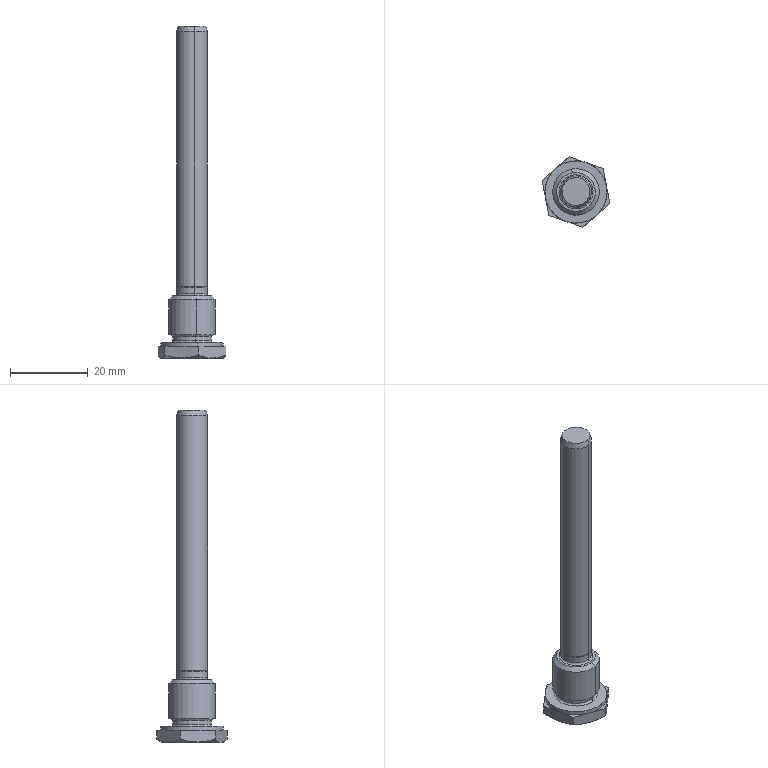Part | SolidWorks | features BaseBody 1 | 1 solid | 46 faces | box 17.462 x 18.14 x 85.5 mm | volume 5617 mm3 | plane 17 | cone 11 | cylinder 10 | torus 8 | commonest cylinder face diameters 7.8 x2 8 x2 10 x2 12 x2 16 x2
STEP:
#1=CARTESIAN_POINT('',(389.341,188.927,-32.5));
#2=VERTEX_POINT('',#1);
#3=CARTESIAN_POINT('',(390.859,181.073,-32.5));
#4=VERTEX_POINT('',#3);
#5=CARTESIAN_POINT('',(390.1,185.,-32.5));
#6=DIRECTION('',(0.,0.,-1.));
#7=DIRECTION('',(0.1897,-0.9818,0.));
#8=AXIS2_PLACEMENT_3D('',#5,#6,#7);
#9=CIRCLE('',#8,4.);
#10=EDGE_CURVE('',#2,#4,#9,.T.);
#11=ORIENTED_EDGE('',*,*,#10,.T.);
#12=CARTESIAN_POINT('',(390.84,181.171,-32.8));
#13=VERTEX_POINT('',#12);
#14=CARTESIAN_POINT('',(390.935,180.68,-32.8));
#15=DIRECTION('',(-0.9818,-0.1897,0.));
#16=DIRECTION('',(0.1897,-0.9818,0.));
#17=AXIS2_PLACEMENT_3D('',#14,#15,#16);
#18=CIRCLE('',#17,0.5);
#19=EDGE_CURVE('',#4,#13,#18,.T.);
#20=ORIENTED_EDGE('',*,*,#19,.T.);
#21=CARTESIAN_POINT('',(389.36,188.829,-32.8));
#22=VERTEX_POINT('',#21);
#23=CARTESIAN_POINT('',(390.1,185.,-32.8));
#24=DIRECTION('',(0.,0.,-1.));
#25=DIRECTION('',(-0.1897,0.9818,0.));
#26=AXIS2_PLACEMENT_3D('',#23,#24,#25);
#27=CIRCLE('',#26,3.9);
#28=EDGE_CURVE('',#22,#13,#27,.T.);
#29=ORIENTED_EDGE('',*,*,#28,.F.);
#30=CARTESIAN_POINT('',(389.265,189.32,-32.8));
#31=DIRECTION('',(0.9818,0.1897,0.));
#32=DIRECTION('',(-0.1897,0.9818,0.));
#33=AXIS2_PLACEMENT_3D('',#30,#31,#32);
#34=CIRCLE('',#33,0.5);
#35=EDGE_CURVE('',#2,#22,#34,.T.);
#36=ORIENTED_EDGE('',*,*,#35,.F.);
#37=EDGE_LOOP('',(#11,#20,#29,#36));
#38=FACE_OUTER_BOUND('',#37,.T.);
#39=CARTESIAN_POINT('',(390.1,185.,-32.8));
#40=DIRECTION('',(0.,0.,1.));
#41=DIRECTION('',(-0.1897,0.9818,0.));
#42=AXIS2_PLACEMENT_3D('',#39,#40,#41);
#43=TOROIDAL_SURFACE('',#42,4.4,0.5);
#44=ADVANCED_FACE('',(#38),#43,.F.);
#45=CARTESIAN_POINT('',(390.84,181.171,-34.5));
#46=VERTEX_POINT('',#45);
#47=CARTESIAN_POINT('',(389.36,188.829,-34.5));
#48=VERTEX_POINT('',#47);
#49=CARTESIAN_POINT('',(390.1,185.,-34.5));
#50=DIRECTION('',(0.,0.,1.));
#51=DIRECTION('',(-0.1897,0.9818,0.));
#52=AXIS2_PLACEMENT_3D('',#49,#50,#51);
#53=CIRCLE('',#52,3.9);
#54=EDGE_CURVE('',#46,#48,#53,.T.);
#55=ORIENTED_EDGE('',*,*,#54,.F.);
#56=CARTESIAN_POINT('',(390.935,180.68,-35.));
#57=VERTEX_POINT('',#56);
#58=CARTESIAN_POINT('',(390.935,180.68,-34.5));
#59=DIRECTION('',(-0.9818,-0.1897,0.));
#60=DIRECTION('',(0.1897,-0.9818,0.));
#61=AXIS2_PLACEMENT_3D('',#58,#59,#60);
#62=CIRCLE('',#61,0.5);
#63=EDGE_CURVE('',#46,#57,#62,.T.);
#64=ORIENTED_EDGE('',*,*,#63,.T.);
#65=CARTESIAN_POINT('',(389.265,189.32,-35.));
#66=VERTEX_POINT('',#65);
#67=CARTESIAN_POINT('',(390.1,185.,-35.));
#68=DIRECTION('',(0.,0.,-1.));
#69=DIRECTION('',(-0.1897,0.9818,0.));
#70=AXIS2_PLACEMENT_3D('',#67,#68,#69);
#71=CIRCLE('',#70,4.4);
#72=EDGE_CURVE('',#66,#57,#71,.T.);
#73=ORIENTED_EDGE('',*,*,#72,.F.);
#74=CARTESIAN_POINT('',(389.265,189.32,-34.5));
#75=DIRECTION('',(0.9818,0.1897,0.));
#76=DIRECTION('',(-0.1897,0.9818,0.));
#77=AXIS2_PLACEMENT_3D('',#74,#75,#76);
#78=CIRCLE('',#77,0.5);
#79=EDGE_CURVE('',#48,#66,#78,.T.);
#80=ORIENTED_EDGE('',*,*,#79,.F.);
#81=EDGE_LOOP('',(#55,#64,#73,#80));
#82=FACE_OUTER_BOUND('',#81,.T.);
#83=CARTESIAN_POINT('',(390.1,185.,-34.5));
#84=DIRECTION('',(0.,0.,1.));
#85=DIRECTION('',(-0.1897,0.9818,0.));
#86=AXIS2_PLACEMENT_3D('',#83,#84,#85);
#87=TOROIDAL_SURFACE('',#86,4.4,0.5);
#88=ADVANCED_FACE('',(#82),#87,.F.);
#89=CARTESIAN_POINT('',(391.143,179.6,-45.));
#90=VERTEX_POINT('',#89);
#91=CARTESIAN_POINT('',(389.057,190.4,-45.));
#92=VERTEX_POINT('',#91);
#93=CARTESIAN_POINT('',(390.1,185.,-45.));
#94=DIRECTION('',(0.,0.,1.));
#95=DIRECTION('',(-0.1897,0.9818,0.));
#96=AXIS2_PLACEMENT_3D('',#93,#94,#95);
#97=CIRCLE('',#96,5.5);
#98=EDGE_CURVE('',#90,#92,#97,.T.);
#99=ORIENTED_EDGE('',*,*,#98,.F.);
#100=CARTESIAN_POINT('',(391.048,180.091,-45.5));
#101=VERTEX_POINT('',#100);
#102=CARTESIAN_POINT('',(391.143,179.6,-45.5));
#103=DIRECTION('',(-0.9818,-0.1897,0.));
#104=DIRECTION('',(0.1897,-0.9818,0.));
#105=AXIS2_PLACEMENT_3D('',#102,#103,#104);
#106=CIRCLE('',#105,0.5);
#107=EDGE_CURVE('',#90,#101,#106,.T.);
#108=ORIENTED_EDGE('',*,*,#107,.T.);
#109=CARTESIAN_POINT('',(389.152,189.909,-45.5));
#110=VERTEX_POINT('',#109);
#111=CARTESIAN_POINT('',(390.1,185.,-45.5));
#112=DIRECTION('',(0.,0.,-1.));
#113=DIRECTION('',(-0.1897,0.9818,0.));
#114=AXIS2_PLACEMENT_3D('',#111,#112,#113);
#115=CIRCLE('',#114,5.);
#116=EDGE_CURVE('',#110,#101,#115,.T.);
#117=ORIENTED_EDGE('',*,*,#116,.F.);
#118=CARTESIAN_POINT('',(389.057,190.4,-45.5));
#119=DIRECTION('',(0.9818,0.1897,0.));
#120=DIRECTION('',(-0.1897,0.9818,0.));
#121=AXIS2_PLACEMENT_3D('',#118,#119,#120);
#122=CIRCLE('',#121,0.5);
#123=EDGE_CURVE('',#92,#110,#122,.T.);
#124=ORIENTED_EDGE('',*,*,#123,.F.);
#125=EDGE_LOOP('',(#99,#108,#117,#124));
#126=FACE_OUTER_BOUND('',#125,.T.);
#127=CARTESIAN_POINT('',(390.1,185.,-45.5));
#128=DIRECTION('',(0.,0.,1.));
#129=DIRECTION('',(-0.1897,0.9818,0.));
#130=AXIS2_PLACEMENT_3D('',#127,#128,#129);
#131=TOROIDAL_SURFACE('',#130,5.5,0.5);
#132=ADVANCED_FACE('',(#126),#131,.F.);
#133=CARTESIAN_POINT('',(391.618,177.145,-51.));
#134=VERTEX_POINT('',#133);
#135=CARTESIAN_POINT('',(387.487,177.439,-51.));
#136=VERTEX_POINT('',#135);
#137=CARTESIAN_POINT('',(390.1,185.,-51.));
#138=DIRECTION('',(0.,0.,-1.));
#139=DIRECTION('',(0.1897,-0.9818,0.));
#140=AXIS2_PLACEMENT_3D('',#137,#138,#139);
#141=CIRCLE('',#140,8.);
#142=EDGE_CURVE('',#134,#136,#141,.T.);
#143=ORIENTED_EDGE('',*,*,#142,.F.);
#144=CARTESIAN_POINT('',(391.852,175.93,-50.285));
#145=VERTEX_POINT('',#144);
#146=CARTESIAN_POINT('',(391.618,177.145,-51.));
#147=DIRECTION('',(0.1643,-0.8503,0.5));
#148=VECTOR('',#147,1000.);
#149=LINE('',#146,#148);
#150=EDGE_CURVE('',#134,#145,#149,.T.);
#151=ORIENTED_EDGE('',*,*,#150,.T.);
#152=CARTESIAN_POINT('',(387.487,177.439,-51.));
#153=CARTESIAN_POINT('',(387.857,177.311,-51.));
#154=CARTESIAN_POINT('',(388.229,177.182,-50.983));
#155=CARTESIAN_POINT('',(388.966,176.928,-50.918));
#156=CARTESIAN_POINT('',(389.331,176.801,-50.869));
#157=CARTESIAN_POINT('',(390.422,176.425,-50.683));
#158=CARTESIAN_POINT('',(391.14,176.176,-50.503));
#159=CARTESIAN_POINT('',(391.852,175.93,-50.285));
#160=B_SPLINE_CURVE_WITH_KNOTS('',3,(#152,#153,#154,#155,#156,#157,#158,#159),.UNSPECIFIED.,.F.,.F.,(4,2,2,4),(0.004674,0.005838,0.007002,0.00933),.UNSPECIFIED.);
#161=EDGE_CURVE('',#136,#145,#160,.T.);
#162=ORIENTED_EDGE('',*,*,#161,.F.);
#163=EDGE_LOOP('',(#143,#151,#162));
#164=FACE_OUTER_BOUND('',#163,.T.);
#165=CARTESIAN_POINT('',(390.1,185.,-51.));
#166=DIRECTION('',(0.,0.,1.));
#167=DIRECTION('',(0.1897,-0.9818,0.));
#168=AXIS2_PLACEMENT_3D('',#165,#166,#167);
#169=CONICAL_SURFACE('',#168,8.,1.047);
#170=ADVANCED_FACE('',(#164),#169,.T.);
#171=CARTESIAN_POINT('',(389.057,190.4,-47.));
#172=VERTEX_POINT('',#171);
#173=CARTESIAN_POINT('',(391.143,179.6,-47.));
#174=VERTEX_POINT('',#173);
#175=CARTESIAN_POINT('',(390.1,185.,-47.));
#176=DIRECTION('',(0.,0.,-1.));
#177=DIRECTION('',(0.1897,-0.9818,0.));
#178=AXIS2_PLACEMENT_3D('',#175,#176,#177);
#179=CIRCLE('',#178,5.5);
#180=EDGE_CURVE('',#172,#174,#179,.T.);
#181=ORIENTED_EDGE('',*,*,#180,.F.);
#182=CARTESIAN_POINT('',(389.152,189.909,-46.5));
#183=VERTEX_POINT('',#182);
#184=CARTESIAN_POINT('',(389.057,190.4,-46.5));
#185=DIRECTION('',(-0.9818,-0.1897,0.));
#186=DIRECTION('',(0.1897,-0.9818,0.));
#187=AXIS2_PLACEMENT_3D('',#184,#185,#186);
#188=CIRCLE('',#187,0.5);
#189=EDGE_CURVE('',#172,#183,#188,.T.);
#190=ORIENTED_EDGE('',*,*,#189,.T.);
#191=CARTESIAN_POINT('',(391.048,180.091,-46.5));
#192=VERTEX_POINT('',#191);
#193=CARTESIAN_POINT('',(390.1,185.,-46.5));
#194=DIRECTION('',(0.,0.,1.));
#195=DIRECTION('',(0.1897,-0.9818,0.));
#196=AXIS2_PLACEMENT_3D('',#193,#194,#195);
#197=CIRCLE('',#196,5.);
#198=EDGE_CURVE('',#192,#183,#197,.T.);
#199=ORIENTED_EDGE('',*,*,#198,.F.);
#200=CARTESIAN_POINT('',(391.143,179.6,-46.5));
#201=DIRECTION('',(0.9818,0.1897,0.));
#202=DIRECTION('',(-0.1897,0.9818,0.));
#203=AXIS2_PLACEMENT_3D('',#200,#201,#202);
#204=CIRCLE('',#203,0.5);
#205=EDGE_CURVE('',#174,#192,#204,.T.);
#206=ORIENTED_EDGE('',*,*,#205,.F.);
#207=EDGE_LOOP('',(#181,#190,#199,#206));
#208=FACE_OUTER_BOUND('',#207,.T.);
#209=CARTESIAN_POINT('',(390.1,185.,-46.5));
#210=DIRECTION('',(0.,0.,-1.));
#211=DIRECTION('',(0.1897,-0.9818,0.));
#212=AXIS2_PLACEMENT_3D('',#209,#210,#211);
#213=TOROIDAL_SURFACE('',#212,5.5,0.5);
#214=ADVANCED_FACE('',(#208),#213,.F.);
#215=CARTESIAN_POINT('',(389.152,189.909,-35.));
#216=VERTEX_POINT('',#215);
#217=CARTESIAN_POINT('',(391.048,180.091,-35.));
#218=VERTEX_POINT('',#217);
#219=CARTESIAN_POINT('',(390.1,185.,-35.));
#220=DIRECTION('',(0.,0.,1.));
#221=DIRECTION('',(-0.1897,0.9818,0.));
#222=AXIS2_PLACEMENT_3D('',#219,#220,#221);
#223=CIRCLE('',#222,5.);
#224=EDGE_CURVE('',#216,#218,#223,.T.);
#225=ORIENTED_EDGE('',*,*,#224,.F.);
#226=CARTESIAN_POINT('',(388.962,190.891,-36.));
#227=VERTEX_POINT('',#226);
#228=CARTESIAN_POINT('',(388.962,190.891,-36.));
#229=DIRECTION('',(-0.1341,0.6943,-0.7071));
#230=VECTOR('',#229,1000.);
#231=LINE('',#228,#230);
#232=EDGE_CURVE('',#216,#227,#231,.T.);
#233=ORIENTED_EDGE('',*,*,#232,.T.);
#234=CARTESIAN_POINT('',(391.238,179.109,-36.));
#235=VERTEX_POINT('',#234);
#236=CARTESIAN_POINT('',(390.1,185.,-36.));
#237=DIRECTION('',(0.,0.,-1.));
#238=DIRECTION('',(-0.1897,0.9818,0.));
#239=AXIS2_PLACEMENT_3D('',#236,#237,#238);
#240=CIRCLE('',#239,6.);
#241=EDGE_CURVE('',#235,#227,#240,.T.);
#242=ORIENTED_EDGE('',*,*,#241,.F.);
#243=CARTESIAN_POINT('',(391.238,179.109,-36.));
#244=DIRECTION('',(0.1341,-0.6943,-0.7071));
#245=VECTOR('',#244,1000.);
#246=LINE('',#243,#245);
#247=EDGE_CURVE('',#218,#235,#246,.T.);
#248=ORIENTED_EDGE('',*,*,#247,.F.);
#249=EDGE_LOOP('',(#225,#233,#242,#248));
#250=FACE_OUTER_BOUND('',#249,.T.);
#251=CARTESIAN_POINT('',(390.1,185.,-36.));
#252=DIRECTION('',(0.,0.,-1.));
#253=DIRECTION('',(0.1897,-0.9818,0.));
#254=AXIS2_PLACEMENT_3D('',#251,#252,#253);
#255=CONICAL_SURFACE('',#254,6.,0.7854);
#256=ADVANCED_FACE('',(#250),#255,.T.);
#257=CARTESIAN_POINT('',(391.618,177.145,-47.));
#258=VERTEX_POINT('',#257);
#259=CARTESIAN_POINT('',(388.582,192.855,-47.));
#260=VERTEX_POINT('',#259);
#261=CARTESIAN_POINT('',(390.1,185.,-47.));
#262=DIRECTION('',(0.,0.,-1.));
#263=DIRECTION('',(0.1897,-0.9818,0.));
#264=AXIS2_PLACEMENT_3D('',#261,#262,#263);
#265=CIRCLE('',#264,8.);
#266=EDGE_CURVE('',#258,#260,#265,.T.);
#267=ORIENTED_EDGE('',*,*,#266,.T.);
#268=CARTESIAN_POINT('',(388.582,192.855,-48.));
#269=VERTEX_POINT('',#268);
#270=CARTESIAN_POINT('',(388.582,192.855,-51.));
#271=DIRECTION('',(0.,0.,-1.));
#272=VECTOR('',#271,1000.);
#273=LINE('',#270,#272);
#274=EDGE_CURVE('',#260,#269,#273,.T.);
#275=ORIENTED_EDGE('',*,*,#274,.T.);
#276=CARTESIAN_POINT('',(384.858,191.044,-48.));
#277=VERTEX_POINT('',#276);
#278=CARTESIAN_POINT('',(390.1,185.,-48.));
#279=DIRECTION('',(0.,0.,-1.));
#280=DIRECTION('',(0.1897,-0.9818,0.));
#281=AXIS2_PLACEMENT_3D('',#278,#279,#280);
#282=CIRCLE('',#281,8.);
#283=EDGE_CURVE('',#277,#269,#282,.T.);
#284=ORIENTED_EDGE('',*,*,#283,.F.);
#285=CARTESIAN_POINT('',(382.245,183.482,-48.));
#286=VERTEX_POINT('',#285);
#287=CARTESIAN_POINT('',(390.1,185.,-48.));
#288=DIRECTION('',(0.,0.,-1.));
#289=DIRECTION('',(0.1897,-0.9818,0.));
#290=AXIS2_PLACEMENT_3D('',#287,#288,#289);
#291=CIRCLE('',#290,8.);
#292=EDGE_CURVE('',#286,#277,#291,.T.);
#293=ORIENTED_EDGE('',*,*,#292,.F.);
#294=CARTESIAN_POINT('',(387.487,177.439,-48.));
#295=VERTEX_POINT('',#294);
#296=CARTESIAN_POINT('',(390.1,185.,-48.));
#297=DIRECTION('',(0.,0.,-1.));
#298=DIRECTION('',(0.1897,-0.9818,0.));
#299=AXIS2_PLACEMENT_3D('',#296,#297,#298);
#300=CIRCLE('',#299,8.);
#301=EDGE_CURVE('',#295,#286,#300,.T.);
#302=ORIENTED_EDGE('',*,*,#301,.F.);
#303=CARTESIAN_POINT('',(391.618,177.145,-48.));
#304=VERTEX_POINT('',#303);
#305=CARTESIAN_POINT('',(390.1,185.,-48.));
#306=DIRECTION('',(0.,0.,-1.));
#307=DIRECTION('',(0.1897,-0.9818,0.));
#308=AXIS2_PLACEMENT_3D('',#305,#306,#307);
#309=CIRCLE('',#308,8.);
#310=EDGE_CURVE('',#304,#295,#309,.T.);
#311=ORIENTED_EDGE('',*,*,#310,.F.);
#312=CARTESIAN_POINT('',(391.618,177.145,-51.));
#313=DIRECTION('',(0.,0.,-1.));
#314=VECTOR('',#313,1000.);
#315=LINE('',#312,#314);
#316=EDGE_CURVE('',#258,#304,#315,.T.);
#317=ORIENTED_EDGE('',*,*,#316,.F.);
#318=EDGE_LOOP('',(#267,#275,#284,#293,#302,#311,#317));
#319=FACE_OUTER_BOUND('',#318,.T.);
#320=CARTESIAN_POINT('',(390.1,185.,-51.));
#321=DIRECTION('',(0.,0.,-1.));
#322=DIRECTION('',(0.1897,-0.9818,0.));
#323=AXIS2_PLACEMENT_3D('',#320,#321,#322);
#324=CYLINDRICAL_SURFACE('',#323,8.);
#325=ADVANCED_FACE('',(#319),#324,.T.);
#326=CARTESIAN_POINT('',(390.1,185.,-45.5));
#327=DIRECTION('',(0.,0.,-1.));
#328=DIRECTION('',(-0.1897,0.9818,0.));
#329=AXIS2_PLACEMENT_3D('',#326,#327,#328);
#330=CIRCLE('',#329,5.);
#331=EDGE_CURVE('',#101,#110,#330,.T.);
#332=ORIENTED_EDGE('',*,*,#331,.T.);
#333=CARTESIAN_POINT('',(389.152,189.909,-51.));
#334=DIRECTION('',(0.,0.,-1.));
#335=VECTOR('',#334,1000.);
#336=LINE('',#333,#335);
#337=EDGE_CURVE('',#110,#183,#336,.T.);
#338=ORIENTED_EDGE('',*,*,#337,.T.);
#339=CARTESIAN_POINT('',(390.1,185.,-46.5));
#340=DIRECTION('',(0.,0.,1.));
#341=DIRECTION('',(0.1897,-0.9818,0.));
#342=AXIS2_PLACEMENT_3D('',#339,#340,#341);
#343=CIRCLE('',#342,5.);
#344=EDGE_CURVE('',#183,#192,#343,.T.);
#345=ORIENTED_EDGE('',*,*,#344,.T.);
#346=CARTESIAN_POINT('',(391.048,180.091,-51.));
#347=DIRECTION('',(0.,0.,-1.));
#348=VECTOR('',#347,1000.);
#349=LINE('',#346,#348);
#350=EDGE_CURVE('',#101,#192,#349,.T.);
#351=ORIENTED_EDGE('',*,*,#350,.F.);
#352=EDGE_LOOP('',(#332,#338,#345,#351));
#353=FACE_OUTER_BOUND('',#352,.T.);
#354=CARTESIAN_POINT('',(390.1,185.,-51.));
#355=DIRECTION('',(0.,0.,-1.));
#356=DIRECTION('',(0.1897,-0.9818,0.));
#357=AXIS2_PLACEMENT_3D('',#354,#355,#356);
#358=CYLINDRICAL_SURFACE('',#357,5.);
#359=ADVANCED_FACE('',(#353),#358,.T.);
#360=ORIENTED_EDGE('',*,*,#241,.T.);
#361=CARTESIAN_POINT('',(388.962,190.891,-45.));
#362=VERTEX_POINT('',#361);
#363=CARTESIAN_POINT('',(388.962,190.891,-51.));
#364=DIRECTION('',(0.,0.,-1.));
#365=VECTOR('',#364,1000.);
#366=LINE('',#363,#365);
#367=EDGE_CURVE('',#227,#362,#366,.T.);
#368=ORIENTED_EDGE('',*,*,#367,.T.);
#369=CARTESIAN_POINT('',(391.238,179.109,-45.));
#370=VERTEX_POINT('',#369);
#371=CARTESIAN_POINT('',(390.1,185.,-45.));
#372=DIRECTION('',(0.,0.,-1.));
#373=DIRECTION('',(0.1897,-0.9818,0.));
#374=AXIS2_PLACEMENT_3D('',#371,#372,#373);
#375=CIRCLE('',#374,6.);
#376=EDGE_CURVE('',#370,#362,#375,.T.);
#377=ORIENTED_EDGE('',*,*,#376,.F.);
#378=CARTESIAN_POINT('',(391.238,179.109,-51.));
#379=DIRECTION('',(0.,0.,-1.));
#380=VECTOR('',#379,1000.);
#381=LINE('',#378,#380);
#382=EDGE_CURVE('',#235,#370,#381,.T.);
#383=ORIENTED_EDGE('',*,*,#382,.F.);
#384=EDGE_LOOP('',(#360,#368,#377,#383));
#385=FACE_OUTER_BOUND('',#384,.T.);
#386=CARTESIAN_POINT('',(390.1,185.,-51.));
#387=DIRECTION('',(0.,0.,-1.));
#388=DIRECTION('',(0.1897,-0.9818,0.));
#389=AXIS2_PLACEMENT_3D('',#386,#387,#388);
#390=CYLINDRICAL_SURFACE('',#389,6.);
#391=ADVANCED_FACE('',(#385),#390,.T.);
#392=CARTESIAN_POINT('',(390.1,185.,-32.8));
#393=DIRECTION('',(0.,0.,-1.));
#394=DIRECTION('',(-0.1897,0.9818,0.));
#395=AXIS2_PLACEMENT_3D('',#392,#393,#394);
#396=CIRCLE('',#395,3.9);
#397=EDGE_CURVE('',#13,#22,#396,.T.);
#398=ORIENTED_EDGE('',*,*,#397,.T.);
#399=CARTESIAN_POINT('',(389.36,188.829,-51.));
#400=DIRECTION('',(0.,0.,-1.));
#401=VECTOR('',#400,1000.);
#402=LINE('',#399,#401);
#403=EDGE_CURVE('',#22,#48,#402,.T.);
#404=ORIENTED_EDGE('',*,*,#403,.T.);
#405=CARTESIAN_POINT('',(390.1,185.,-34.5));
#406=DIRECTION('',(0.,0.,1.));
#407=DIRECTION('',(-0.1897,0.9818,0.));
#408=AXIS2_PLACEMENT_3D('',#405,#406,#407);
#409=CIRCLE('',#408,3.9);
#410=EDGE_CURVE('',#48,#46,#409,.T.);
#411=ORIENTED_EDGE('',*,*,#410,.T.);
#412=CARTESIAN_POINT('',(390.84,181.171,-51.));
#413=DIRECTION('',(0.,0.,-1.));
#414=VECTOR('',#413,1000.);
#415=LINE('',#412,#414);
#416=EDGE_CURVE('',#13,#46,#415,.T.);
#417=ORIENTED_EDGE('',*,*,#416,.F.);
#418=EDGE_LOOP('',(#398,#404,#411,#417));
#419=FACE_OUTER_BOUND('',#418,.T.);
#420=CARTESIAN_POINT('',(390.1,185.,-51.));
#421=DIRECTION('',(0.,0.,-1.));
#422=DIRECTION('',(0.1897,-0.9818,0.));
#423=AXIS2_PLACEMENT_3D('',#420,#421,#422);
#424=CYLINDRICAL_SURFACE('',#423,3.9);
#425=ADVANCED_FACE('',(#419),#424,.T.);
#426=CARTESIAN_POINT('',(390.859,181.073,33.));
#427=VERTEX_POINT('',#426);
#428=CARTESIAN_POINT('',(389.341,188.927,33.));
#429=VERTEX_POINT('',#428);
#430=CARTESIAN_POINT('',(390.1,185.,33.));
#431=DIRECTION('',(0.,0.,-1.));
#432=DIRECTION('',(0.1897,-0.9818,0.));
#433=AXIS2_PLACEMENT_3D('',#430,#431,#432);
#434=CIRCLE('',#433,4.);
#435=EDGE_CURVE('',#427,#429,#434,.T.);
#436=ORIENTED_EDGE('',*,*,#435,.T.);
#437=CARTESIAN_POINT('',(389.341,188.927,-51.));
#438=DIRECTION('',(0.,0.,-1.));
#439=VECTOR('',#438,1000.);
#440=LINE('',#437,#439);
#441=EDGE_CURVE('',#429,#2,#440,.T.);
#442=ORIENTED_EDGE('',*,*,#441,.T.);
#443=CARTESIAN_POINT('',(390.1,185.,-32.5));
#444=DIRECTION('',(0.,0.,-1.));
#445=DIRECTION('',(0.1897,-0.9818,0.));
#446=AXIS2_PLACEMENT_3D('',#443,#444,#445);
#447=CIRCLE('',#446,4.);
#448=EDGE_CURVE('',#4,#2,#447,.T.);
#449=ORIENTED_EDGE('',*,*,#448,.F.);
#450=CARTESIAN_POINT('',(390.859,181.073,-51.));
#451=DIRECTION('',(0.,0.,-1.));
#452=VECTOR('',#451,1000.);
#453=LINE('',#450,#452);
#454=EDGE_CURVE('',#427,#4,#453,.T.);
#455=ORIENTED_EDGE('',*,*,#454,.F.);
#456=EDGE_LOOP('',(#436,#442,#449,#455));
#457=FACE_OUTER_BOUND('',#456,.T.);
#458=CARTESIAN_POINT('',(390.1,185.,-51.));
#459=DIRECTION('',(0.,0.,-1.));
#460=DIRECTION('',(0.1897,-0.9818,0.));
#461=AXIS2_PLACEMENT_3D('',#458,#459,#460);
#462=CYLINDRICAL_SURFACE('',#461,4.);
#463=ADVANCED_FACE('',(#457),#462,.T.);
#464=CARTESIAN_POINT('',(390.783,181.467,34.5));
#465=VERTEX_POINT('',#464);
#466=CARTESIAN_POINT('',(389.417,188.533,34.5));
#467=VERTEX_POINT('',#466);
#468=CARTESIAN_POINT('',(390.1,185.,34.5));
#469=DIRECTION('',(0.,0.,-1.));
#470=DIRECTION('',(0.1897,-0.9818,0.));
#471=AXIS2_PLACEMENT_3D('',#468,#469,#470);
#472=CIRCLE('',#471,3.598);
#473=EDGE_CURVE('',#465,#467,#472,.T.);
#474=ORIENTED_EDGE('',*,*,#473,.T.);
#475=CARTESIAN_POINT('',(389.417,188.533,34.5));
#476=DIRECTION('',(-0.0491,0.2541,-0.9659));
#477=VECTOR('',#476,1000.);
#478=LINE('',#475,#477);
#479=EDGE_CURVE('',#467,#429,#478,.T.);
#480=ORIENTED_EDGE('',*,*,#479,.T.);
#481=ORIENTED_EDGE('',*,*,#435,.F.);
#482=CARTESIAN_POINT('',(390.783,181.467,34.5));
#483=DIRECTION('',(0.0491,-0.2541,-0.9659));
#484=VECTOR('',#483,1000.);
#485=LINE('',#482,#484);
#486=EDGE_CURVE('',#465,#427,#485,.T.);
#487=ORIENTED_EDGE('',*,*,#486,.F.);
#488=EDGE_LOOP('',(#474,#480,#481,#487));
#489=FACE_OUTER_BOUND('',#488,.T.);
#490=CARTESIAN_POINT('',(390.1,185.,34.5));
#491=DIRECTION('',(0.,0.,-1.));
#492=DIRECTION('',(0.1897,-0.9818,0.));
#493=AXIS2_PLACEMENT_3D('',#490,#491,#492);
#494=CONICAL_SURFACE('',#493,3.598,0.2618);
#495=ADVANCED_FACE('',(#489),#494,.T.);
#496=CARTESIAN_POINT('',(391.852,175.93,-48.));
#497=VERTEX_POINT('',#496);
#498=CARTESIAN_POINT('',(391.852,175.93,-48.));
#499=DIRECTION('',(0.,0.,-1.));
#500=VECTOR('',#499,1000.);
#501=LINE('',#498,#500);
#502=EDGE_CURVE('',#497,#145,#501,.T.);
#503=ORIENTED_EDGE('',*,*,#502,.T.);
#504=CARTESIAN_POINT('',(395.342,178.956,-51.));
#505=VERTEX_POINT('',#504);
#506=CARTESIAN_POINT('',(391.852,175.93,-50.285));
#507=CARTESIAN_POINT('',(392.423,176.425,-50.504));
#508=CARTESIAN_POINT('',(392.998,176.924,-50.683));
#509=CARTESIAN_POINT('',(394.16,177.932,-50.932));
#510=CARTESIAN_POINT('',(394.747,178.441,-51.));
#511=CARTESIAN_POINT('',(395.342,178.956,-51.));
#512=B_SPLINE_CURVE_WITH_KNOTS('',3,(#506,#507,#508,#509,#510,#511),.UNSPECIFIED.,.F.,.F.,(4,2,4),(0.000000238,0.002337,0.004674),.UNSPECIFIED.);
#513=EDGE_CURVE('',#145,#505,#512,.T.);
#514=ORIENTED_EDGE('',*,*,#513,.T.);
#515=CARTESIAN_POINT('',(398.831,181.983,-50.285));
#516=VERTEX_POINT('',#515);
#517=CARTESIAN_POINT('',(395.342,178.956,-51.));
#518=CARTESIAN_POINT('',(395.638,179.213,-51.));
#519=CARTESIAN_POINT('',(395.935,179.471,-50.983));
#520=CARTESIAN_POINT('',(396.524,179.981,-50.918));
#521=CARTESIAN_POINT('',(396.816,180.235,-50.869));
#522=CARTESIAN_POINT('',(397.687,180.991,-50.683));
#523=CARTESIAN_POINT('',(398.262,181.489,-50.503));
#524=CARTESIAN_POINT('',(398.831,181.983,-50.285));
#525=B_SPLINE_CURVE_WITH_KNOTS('',3,(#517,#518,#519,#520,#521,#522,#523,#524),.UNSPECIFIED.,.F.,.F.,(4,2,2,4),(0.004674,0.005838,0.007002,0.00933),.UNSPECIFIED.);
#526=EDGE_CURVE('',#505,#516,#525,.T.);
#527=ORIENTED_EDGE('',*,*,#526,.T.);
#528=CARTESIAN_POINT('',(398.831,181.983,-48.));
#529=VERTEX_POINT('',#528);
#530=CARTESIAN_POINT('',(398.831,181.983,-48.));
#531=DIRECTION('',(0.,0.,-1.));
#532=VECTOR('',#531,1000.);
#533=LINE('',#530,#532);
#534=EDGE_CURVE('',#529,#516,#533,.T.);
#535=ORIENTED_EDGE('',*,*,#534,.F.);
#536=CARTESIAN_POINT('',(395.342,178.956,-48.));
#537=VERTEX_POINT('',#536);
#538=CARTESIAN_POINT('',(398.831,181.983,-48.));
#539=DIRECTION('',(-0.7555,-0.6552,0.));
#540=VECTOR('',#539,1000.);
#541=LINE('',#538,#540);
#542=EDGE_CURVE('',#529,#537,#541,.T.);
#543=ORIENTED_EDGE('',*,*,#542,.T.);
#544=CARTESIAN_POINT('',(398.831,181.983,-48.));
#545=DIRECTION('',(-0.7555,-0.6552,0.));
#546=VECTOR('',#545,1000.);
#547=LINE('',#544,#546);
#548=EDGE_CURVE('',#537,#497,#547,.T.);
#549=ORIENTED_EDGE('',*,*,#548,.T.);
#550=EDGE_LOOP('',(#503,#514,#527,#535,#543,#549));
#551=FACE_OUTER_BOUND('',#550,.T.);
#552=CARTESIAN_POINT('',(398.831,181.983,-48.));
#553=DIRECTION('',(0.6552,-0.7555,0.));
#554=DIRECTION('',(-0.7555,-0.6552,0.));
#555=AXIS2_PLACEMENT_3D('',#552,#553,#554);
#556=PLANE('',#555);
#557=ADVANCED_FACE('',(#551),#556,.T.);
#558=ORIENTED_EDGE('',*,*,#534,.T.);
#559=CARTESIAN_POINT('',(397.955,186.518,-51.));
#560=VERTEX_POINT('',#559);
#561=CARTESIAN_POINT('',(398.831,181.983,-50.285));
#562=CARTESIAN_POINT('',(398.689,182.716,-50.501));
#563=CARTESIAN_POINT('',(398.546,183.459,-50.681));
#564=CARTESIAN_POINT('',(398.326,184.594,-50.868));
#565=CARTESIAN_POINT('',(398.253,184.976,-50.917));
#566=CARTESIAN_POINT('',(398.104,185.747,-50.983));
#567=CARTESIAN_POINT('',(398.029,186.134,-51.));
#568=CARTESIAN_POINT('',(397.955,186.518,-51.));
#569=B_SPLINE_CURVE_WITH_KNOTS('',3,(#561,#562,#563,#564,#565,#566,#567,#568),.UNSPECIFIED.,.F.,.F.,(4,2,2,4),(0.02201,0.02435,0.02552,0.02669),.UNSPECIFIED.);
#570=EDGE_CURVE('',#516,#560,#569,.T.);
#571=ORIENTED_EDGE('',*,*,#570,.T.);
#572=CARTESIAN_POINT('',(397.079,191.052,-50.285));
#573=VERTEX_POINT('',#572);
#574=CARTESIAN_POINT('',(397.955,186.518,-51.));
#575=CARTESIAN_POINT('',(397.806,187.285,-51.));
#576=CARTESIAN_POINT('',(397.659,188.046,-50.933));
#577=CARTESIAN_POINT('',(397.367,189.559,-50.684));
#578=CARTESIAN_POINT('',(397.221,190.314,-50.503));
#579=CARTESIAN_POINT('',(397.079,191.052,-50.285));
#580=B_SPLINE_CURVE_WITH_KNOTS('',3,(#574,#575,#576,#577,#578,#579),.UNSPECIFIED.,.F.,.F.,(4,2,4),(0.02669,0.02903,0.03137),.UNSPECIFIED.);
#581=EDGE_CURVE('',#560,#573,#580,.T.);
#582=ORIENTED_EDGE('',*,*,#581,.T.);
#583=CARTESIAN_POINT('',(397.079,191.052,-48.));
#584=VERTEX_POINT('',#583);
#585=CARTESIAN_POINT('',(397.079,191.052,-48.));
#586=DIRECTION('',(0.,0.,-1.));
#587=VECTOR('',#586,1000.);
#588=LINE('',#585,#587);
#589=EDGE_CURVE('',#584,#573,#588,.T.);
#590=ORIENTED_EDGE('',*,*,#589,.F.);
#591=CARTESIAN_POINT('',(397.955,186.518,-48.));
#592=VERTEX_POINT('',#591);
#593=CARTESIAN_POINT('',(397.079,191.052,-48.));
#594=DIRECTION('',(0.1897,-0.9818,0.));
#595=VECTOR('',#594,1000.);
#596=LINE('',#593,#595);
#597=EDGE_CURVE('',#584,#592,#596,.T.);
#598=ORIENTED_EDGE('',*,*,#597,.T.);
#599=CARTESIAN_POINT('',(397.079,191.052,-48.));
#600=DIRECTION('',(0.1897,-0.9818,0.));
#601=VECTOR('',#600,1000.);
#602=LINE('',#599,#601);
#603=EDGE_CURVE('',#592,#529,#602,.T.);
#604=ORIENTED_EDGE('',*,*,#603,.T.);
#605=EDGE_LOOP('',(#558,#571,#582,#590,#598,#604));
#606=FACE_OUTER_BOUND('',#605,.T.);
#607=CARTESIAN_POINT('',(397.079,191.052,-48.));
#608=DIRECTION('',(0.9818,0.1897,0.));
#609=DIRECTION('',(0.1897,-0.9818,0.));
#610=AXIS2_PLACEMENT_3D('',#607,#608,#609);
#611=PLANE('',#610);
#612=ADVANCED_FACE('',(#606),#611,.T.);
#613=ORIENTED_EDGE('',*,*,#589,.T.);
#614=CARTESIAN_POINT('',(392.713,192.561,-51.));
#615=VERTEX_POINT('',#614);
#616=CARTESIAN_POINT('',(397.079,191.052,-50.285));
#617=CARTESIAN_POINT('',(396.364,191.299,-50.504));
#618=CARTESIAN_POINT('',(395.645,191.548,-50.683));
#619=CARTESIAN_POINT('',(394.191,192.05,-50.932));
#620=CARTESIAN_POINT('',(393.457,192.304,-51.));
#621=CARTESIAN_POINT('',(392.713,192.561,-51.));
#622=B_SPLINE_CURVE_WITH_KNOTS('',3,(#616,#617,#618,#619,#620,#621),.UNSPECIFIED.,.F.,.F.,(4,2,4),(0.000000238,0.002337,0.004674),.UNSPECIFIED.);
#623=EDGE_CURVE('',#573,#615,#622,.T.);
#624=ORIENTED_EDGE('',*,*,#623,.T.);
#625=CARTESIAN_POINT('',(388.348,194.07,-50.285));
#626=VERTEX_POINT('',#625);
#627=CARTESIAN_POINT('',(392.713,192.561,-51.));
#628=CARTESIAN_POINT('',(392.343,192.689,-51.));
#629=CARTESIAN_POINT('',(391.971,192.818,-50.983));
#630=CARTESIAN_POINT('',(391.234,193.072,-50.918));
#631=CARTESIAN_POINT('',(390.869,193.199,-50.869));
#632=CARTESIAN_POINT('',(389.778,193.575,-50.683));
#633=CARTESIAN_POINT('',(389.06,193.824,-50.503));
#634=CARTESIAN_POINT('',(388.348,194.07,-50.285));
#635=B_SPLINE_CURVE_WITH_KNOTS('',3,(#627,#628,#629,#630,#631,#632,#633,#634),.UNSPECIFIED.,.F.,.F.,(4,2,2,4),(0.004674,0.005838,0.007002,0.00933),.UNSPECIFIED.);
#636=EDGE_CURVE('',#615,#626,#635,.T.);
#637=ORIENTED_EDGE('',*,*,#636,.T.);
#638=CARTESIAN_POINT('',(388.348,194.07,-48.));
#639=VERTEX_POINT('',#638);
#640=CARTESIAN_POINT('',(388.348,194.07,-48.));
#641=DIRECTION('',(0.,0.,-1.));
#642=VECTOR('',#641,1000.);
#643=LINE('',#640,#642);
#644=EDGE_CURVE('',#639,#626,#643,.T.);
#645=ORIENTED_EDGE('',*,*,#644,.F.);
#646=CARTESIAN_POINT('',(392.713,192.561,-48.));
#647=VERTEX_POINT('',#646);
#648=CARTESIAN_POINT('',(388.348,194.07,-48.));
#649=DIRECTION('',(0.9451,-0.3266,0.));
#650=VECTOR('',#649,1000.);
#651=LINE('',#648,#650);
#652=EDGE_CURVE('',#639,#647,#651,.T.);
#653=ORIENTED_EDGE('',*,*,#652,.T.);
#654=CARTESIAN_POINT('',(388.348,194.07,-48.));
#655=DIRECTION('',(0.9451,-0.3266,0.));
#656=VECTOR('',#655,1000.);
#657=LINE('',#654,#656);
#658=EDGE_CURVE('',#647,#584,#657,.T.);
#659=ORIENTED_EDGE('',*,*,#658,.T.);
#660=EDGE_LOOP('',(#613,#624,#637,#645,#653,#659));
#661=FACE_OUTER_BOUND('',#660,.T.);
#662=CARTESIAN_POINT('',(388.348,194.07,-48.));
#663=DIRECTION('',(0.3266,0.9451,0.));
#664=DIRECTION('',(0.9451,-0.3266,0.));
#665=AXIS2_PLACEMENT_3D('',#662,#663,#664);
#666=PLANE('',#665);
#667=ADVANCED_FACE('',(#661),#666,.T.);
#668=ORIENTED_EDGE('',*,*,#644,.T.);
#669=CARTESIAN_POINT('',(384.858,191.044,-51.));
#670=VERTEX_POINT('',#669);
#671=CARTESIAN_POINT('',(388.348,194.07,-50.285));
#672=CARTESIAN_POINT('',(387.777,193.575,-50.504));
#673=CARTESIAN_POINT('',(387.202,193.076,-50.683));
#674=CARTESIAN_POINT('',(386.04,192.068,-50.932));
#675=CARTESIAN_POINT('',(385.453,191.559,-51.));
#676=CARTESIAN_POINT('',(384.858,191.044,-51.));
#677=B_SPLINE_CURVE_WITH_KNOTS('',3,(#671,#672,#673,#674,#675,#676),.UNSPECIFIED.,.F.,.F.,(4,2,4),(0.000000238,0.002337,0.004674),.UNSPECIFIED.);
#678=EDGE_CURVE('',#626,#670,#677,.T.);
#679=ORIENTED_EDGE('',*,*,#678,.T.);
#680=CARTESIAN_POINT('',(381.369,188.017,-50.285));
#681=VERTEX_POINT('',#680);
#682=CARTESIAN_POINT('',(384.858,191.044,-51.));
#683=CARTESIAN_POINT('',(384.562,190.787,-51.));
#684=CARTESIAN_POINT('',(384.265,190.529,-50.983));
#685=CARTESIAN_POINT('',(383.676,190.019,-50.918));
#686=CARTESIAN_POINT('',(383.384,189.765,-50.869));
#687=CARTESIAN_POINT('',(382.513,189.009,-50.683));
#688=CARTESIAN_POINT('',(381.938,188.511,-50.503));
#689=CARTESIAN_POINT('',(381.369,188.017,-50.285));
#690=B_SPLINE_CURVE_WITH_KNOTS('',3,(#682,#683,#684,#685,#686,#687,#688,#689),.UNSPECIFIED.,.F.,.F.,(4,2,2,4),(0.004674,0.005838,0.007002,0.00933),.UNSPECIFIED.);
#691=EDGE_CURVE('',#670,#681,#690,.T.);
#692=ORIENTED_EDGE('',*,*,#691,.T.);
#693=CARTESIAN_POINT('',(381.369,188.017,-48.));
#694=VERTEX_POINT('',#693);
#695=CARTESIAN_POINT('',(381.369,188.017,-48.));
#696=DIRECTION('',(0.,0.,-1.));
#697=VECTOR('',#696,1000.);
#698=LINE('',#695,#697);
#699=EDGE_CURVE('',#694,#681,#698,.T.);
#700=ORIENTED_EDGE('',*,*,#699,.F.);
#701=CARTESIAN_POINT('',(381.369,188.017,-48.));
#702=DIRECTION('',(0.7555,0.6552,0.));
#703=VECTOR('',#702,1000.);
#704=LINE('',#701,#703);
#705=EDGE_CURVE('',#694,#277,#704,.T.);
#706=ORIENTED_EDGE('',*,*,#705,.T.);
#707=CARTESIAN_POINT('',(381.369,188.017,-48.));
#708=DIRECTION('',(0.7555,0.6552,0.));
#709=VECTOR('',#708,1000.);
#710=LINE('',#707,#709);
#711=EDGE_CURVE('',#277,#639,#710,.T.);
#712=ORIENTED_EDGE('',*,*,#711,.T.);
#713=EDGE_LOOP('',(#668,#679,#692,#700,#706,#712));
#714=FACE_OUTER_BOUND('',#713,.T.);
#715=CARTESIAN_POINT('',(381.369,188.017,-48.));
#716=DIRECTION('',(-0.6552,0.7555,0.));
#717=DIRECTION('',(0.7555,0.6552,0.));
#718=AXIS2_PLACEMENT_3D('',#715,#716,#717);
#719=PLANE('',#718);
#720=ADVANCED_FACE('',(#714),#719,.T.);
#721=ORIENTED_EDGE('',*,*,#699,.T.);
#722=CARTESIAN_POINT('',(382.245,183.482,-51.));
#723=VERTEX_POINT('',#722);
#724=CARTESIAN_POINT('',(381.369,188.017,-50.285));
#725=CARTESIAN_POINT('',(381.512,187.279,-50.503));
#726=CARTESIAN_POINT('',(381.658,186.524,-50.684));
#727=CARTESIAN_POINT('',(381.95,185.011,-50.933));
#728=CARTESIAN_POINT('',(382.097,184.25,-51.));
#729=CARTESIAN_POINT('',(382.245,183.482,-51.));
#730=B_SPLINE_CURVE_WITH_KNOTS('',3,(#724,#725,#726,#727,#728,#729),.UNSPECIFIED.,.F.,.F.,(4,2,4),(0.008596,0.01093,0.01327),.UNSPECIFIED.);
#731=EDGE_CURVE('',#681,#723,#730,.T.);
#732=ORIENTED_EDGE('',*,*,#731,.T.);
#733=CARTESIAN_POINT('',(383.121,178.948,-50.285));
#734=VERTEX_POINT('',#733);
#735=CARTESIAN_POINT('',(382.245,183.482,-51.));
#736=CARTESIAN_POINT('',(382.319,183.098,-51.));
#737=CARTESIAN_POINT('',(382.394,182.712,-50.983));
#738=CARTESIAN_POINT('',(382.543,181.94,-50.917));
#739=CARTESIAN_POINT('',(382.617,181.559,-50.868));
#740=CARTESIAN_POINT('',(382.836,180.424,-50.681));
#741=CARTESIAN_POINT('',(382.98,179.681,-50.501));
#742=CARTESIAN_POINT('',(383.121,178.948,-50.285));
#743=B_SPLINE_CURVE_WITH_KNOTS('',3,(#735,#736,#737,#738,#739,#740,#741,#742),.UNSPECIFIED.,.F.,.F.,(4,2,2,4),(0.01327,0.01444,0.01561,0.01795),.UNSPECIFIED.);
#744=EDGE_CURVE('',#723,#734,#743,.T.);
#745=ORIENTED_EDGE('',*,*,#744,.T.);
#746=CARTESIAN_POINT('',(383.121,178.948,-48.));
#747=VERTEX_POINT('',#746);
#748=CARTESIAN_POINT('',(383.121,178.948,-48.));
#749=DIRECTION('',(0.,0.,-1.));
#750=VECTOR('',#749,1000.);
#751=LINE('',#748,#750);
#752=EDGE_CURVE('',#747,#734,#751,.T.);
#753=ORIENTED_EDGE('',*,*,#752,.F.);
#754=CARTESIAN_POINT('',(383.121,178.948,-48.));
#755=DIRECTION('',(-0.1897,0.9818,0.));
#756=VECTOR('',#755,1000.);
#757=LINE('',#754,#756);
#758=EDGE_CURVE('',#747,#286,#757,.T.);
#759=ORIENTED_EDGE('',*,*,#758,.T.);
#760=CARTESIAN_POINT('',(383.121,178.948,-48.));
#761=DIRECTION('',(-0.1897,0.9818,0.));
#762=VECTOR('',#761,1000.);
#763=LINE('',#760,#762);
#764=EDGE_CURVE('',#286,#694,#763,.T.);
#765=ORIENTED_EDGE('',*,*,#764,.T.);
#766=EDGE_LOOP('',(#721,#732,#745,#753,#759,#765));
#767=FACE_OUTER_BOUND('',#766,.T.);
#768=CARTESIAN_POINT('',(383.121,178.948,-48.));
#769=DIRECTION('',(-0.9818,-0.1897,0.));
#770=DIRECTION('',(-0.1897,0.9818,0.));
#771=AXIS2_PLACEMENT_3D('',#768,#769,#770);
#772=PLANE('',#771);
#773=ADVANCED_FACE('',(#767),#772,.T.);
#774=ORIENTED_EDGE('',*,*,#752,.T.);
#775=CARTESIAN_POINT('',(383.121,178.948,-50.285));
#776=CARTESIAN_POINT('',(383.836,178.701,-50.504));
#777=CARTESIAN_POINT('',(384.555,178.452,-50.683));
#778=CARTESIAN_POINT('',(386.009,177.95,-50.932));
#779=CARTESIAN_POINT('',(386.743,177.696,-51.));
#780=CARTESIAN_POINT('',(387.487,177.439,-51.));
#781=B_SPLINE_CURVE_WITH_KNOTS('',3,(#775,#776,#777,#778,#779,#780),.UNSPECIFIED.,.F.,.F.,(4,2,4),(0.000000238,0.002337,0.004674),.UNSPECIFIED.);
#782=EDGE_CURVE('',#734,#136,#781,.T.);
#783=ORIENTED_EDGE('',*,*,#782,.T.);
#784=ORIENTED_EDGE('',*,*,#161,.T.);
#785=ORIENTED_EDGE('',*,*,#502,.F.);
#786=CARTESIAN_POINT('',(391.852,175.93,-48.));
#787=DIRECTION('',(-0.9451,0.3266,0.));
#788=VECTOR('',#787,1000.);
#789=LINE('',#786,#788);
#790=EDGE_CURVE('',#497,#295,#789,.T.);
#791=ORIENTED_EDGE('',*,*,#790,.T.);
#792=CARTESIAN_POINT('',(391.852,175.93,-48.));
#793=DIRECTION('',(-0.9451,0.3266,0.));
#794=VECTOR('',#793,1000.);
#795=LINE('',#792,#794);
#796=EDGE_CURVE('',#295,#747,#795,.T.);
#797=ORIENTED_EDGE('',*,*,#796,.T.);
#798=EDGE_LOOP('',(#774,#783,#784,#785,#791,#797));
#799=FACE_OUTER_BOUND('',#798,.T.);
#800=CARTESIAN_POINT('',(391.852,175.93,-48.));
#801=DIRECTION('',(-0.3266,-0.9451,0.));
#802=DIRECTION('',(-0.9451,0.3266,0.));
#803=AXIS2_PLACEMENT_3D('',#800,#801,#802);
#804=PLANE('',#803);
#805=ADVANCED_FACE('',(#799),#804,.T.);
#806=ORIENTED_EDGE('',*,*,#796,.F.);
#807=ORIENTED_EDGE('',*,*,#301,.T.);
#808=ORIENTED_EDGE('',*,*,#758,.F.);
#809=EDGE_LOOP('',(#806,#807,#808));
#810=FACE_OUTER_BOUND('',#809,.T.);
#811=CARTESIAN_POINT('',(391.852,175.93,-48.));
#812=DIRECTION('',(0.,0.,-1.));
#813=DIRECTION('',(0.1897,-0.9818,0.));
#814=AXIS2_PLACEMENT_3D('',#811,#812,#813);
#815=PLANE('',#814);
#816=ADVANCED_FACE('',(#810),#815,.F.);
#817=ORIENTED_EDGE('',*,*,#764,.F.);
#818=ORIENTED_EDGE('',*,*,#292,.T.);
#819=ORIENTED_EDGE('',*,*,#705,.F.);
#820=EDGE_LOOP('',(#817,#818,#819));
#821=FACE_OUTER_BOUND('',#820,.T.);
#822=CARTESIAN_POINT('',(391.852,175.93,-48.));
#823=DIRECTION('',(0.,0.,-1.));
#824=DIRECTION('',(0.1897,-0.9818,0.));
#825=AXIS2_PLACEMENT_3D('',#822,#823,#824);
#826=PLANE('',#825);
#827=ADVANCED_FACE('',(#821),#826,.F.);
#828=ORIENTED_EDGE('',*,*,#711,.F.);
#829=ORIENTED_EDGE('',*,*,#283,.T.);
#830=CARTESIAN_POINT('',(390.1,185.,-48.));
#831=DIRECTION('',(0.,0.,-1.));
#832=DIRECTION('',(0.1897,-0.9818,0.));
#833=AXIS2_PLACEMENT_3D('',#830,#831,#832);
#834=CIRCLE('',#833,8.);
#835=EDGE_CURVE('',#269,#647,#834,.T.);
#836=ORIENTED_EDGE('',*,*,#835,.T.);
#837=ORIENTED_EDGE('',*,*,#652,.F.);
#838=EDGE_LOOP('',(#828,#829,#836,#837));
#839=FACE_OUTER_BOUND('',#838,.T.);
#840=CARTESIAN_POINT('',(391.852,175.93,-48.));
#841=DIRECTION('',(0.,0.,-1.));
#842=DIRECTION('',(0.1897,-0.9818,0.));
#843=AXIS2_PLACEMENT_3D('',#840,#841,#842);
#844=PLANE('',#843);
#845=ADVANCED_FACE('',(#839),#844,.F.);
#846=ORIENTED_EDGE('',*,*,#658,.F.);
#847=CARTESIAN_POINT('',(390.1,185.,-48.));
#848=DIRECTION('',(0.,0.,-1.));
#849=DIRECTION('',(0.1897,-0.9818,0.));
#850=AXIS2_PLACEMENT_3D('',#847,#848,#849);
#851=CIRCLE('',#850,8.);
#852=EDGE_CURVE('',#647,#592,#851,.T.);
#853=ORIENTED_EDGE('',*,*,#852,.T.);
#854=ORIENTED_EDGE('',*,*,#597,.F.);
#855=EDGE_LOOP('',(#846,#853,#854));
#856=FACE_OUTER_BOUND('',#855,.T.);
#857=CARTESIAN_POINT('',(391.852,175.93,-48.));
#858=DIRECTION('',(0.,0.,-1.));
#859=DIRECTION('',(0.1897,-0.9818,0.));
#860=AXIS2_PLACEMENT_3D('',#857,#858,#859);
#861=PLANE('',#860);
#862=ADVANCED_FACE('',(#856),#861,.F.);
#863=ORIENTED_EDGE('',*,*,#603,.F.);
#864=CARTESIAN_POINT('',(390.1,185.,-48.));
#865=DIRECTION('',(0.,0.,-1.));
#866=DIRECTION('',(0.1897,-0.9818,0.));
#867=AXIS2_PLACEMENT_3D('',#864,#865,#866);
#868=CIRCLE('',#867,8.);
#869=EDGE_CURVE('',#592,#537,#868,.T.);
#870=ORIENTED_EDGE('',*,*,#869,.T.);
#871=ORIENTED_EDGE('',*,*,#542,.F.);
#872=EDGE_LOOP('',(#863,#870,#871));
#873=FACE_OUTER_BOUND('',#872,.T.);
#874=CARTESIAN_POINT('',(391.852,175.93,-48.));
#875=DIRECTION('',(0.,0.,-1.));
#876=DIRECTION('',(0.1897,-0.9818,0.));
#877=AXIS2_PLACEMENT_3D('',#874,#875,#876);
#878=PLANE('',#877);
#879=ADVANCED_FACE('',(#873),#878,.F.);
#880=ORIENTED_EDGE('',*,*,#548,.F.);
#881=CARTESIAN_POINT('',(390.1,185.,-48.));
#882=DIRECTION('',(0.,0.,-1.));
#883=DIRECTION('',(0.1897,-0.9818,0.));
#884=AXIS2_PLACEMENT_3D('',#881,#882,#883);
#885=CIRCLE('',#884,8.);
#886=EDGE_CURVE('',#537,#304,#885,.T.);
#887=ORIENTED_EDGE('',*,*,#886,.T.);
#888=ORIENTED_EDGE('',*,*,#310,.T.);
#889=ORIENTED_EDGE('',*,*,#790,.F.);
#890=EDGE_LOOP('',(#880,#887,#888,#889));
#891=FACE_OUTER_BOUND('',#890,.T.);
#892=CARTESIAN_POINT('',(391.852,175.93,-48.));
#893=DIRECTION('',(0.,0.,-1.));
#894=DIRECTION('',(0.1897,-0.9818,0.));
#895=AXIS2_PLACEMENT_3D('',#892,#893,#894);
#896=PLANE('',#895);
#897=ADVANCED_FACE('',(#891),#896,.F.);
#898=ORIENTED_EDGE('',*,*,#473,.F.);
#899=CARTESIAN_POINT('',(390.1,185.,34.5));
#900=DIRECTION('',(0.,0.,-1.));
#901=DIRECTION('',(0.1897,-0.9818,0.));
#902=AXIS2_PLACEMENT_3D('',#899,#900,#901);
#903=CIRCLE('',#902,3.598);
#904=EDGE_CURVE('',#467,#465,#903,.T.);
#905=ORIENTED_EDGE('',*,*,#904,.F.);
#906=EDGE_LOOP('',(#898,#905));
#907=FACE_OUTER_BOUND('',#906,.T.);
#908=CARTESIAN_POINT('',(377.084,252.371,34.5));
#909=DIRECTION('',(0.,0.,1.));
#910=DIRECTION('',(-0.1897,0.9818,0.));
#911=AXIS2_PLACEMENT_3D('',#908,#909,#910);
#912=PLANE('',#911);
#913=ADVANCED_FACE('',(#907),#912,.T.);
#914=ORIENTED_EDGE('',*,*,#479,.F.);
#915=ORIENTED_EDGE('',*,*,#904,.T.);
#916=ORIENTED_EDGE('',*,*,#486,.T.);
#917=CARTESIAN_POINT('',(390.1,185.,33.));
#918=DIRECTION('',(0.,0.,-1.));
#919=DIRECTION('',(0.1897,-0.9818,0.));
#920=AXIS2_PLACEMENT_3D('',#917,#918,#919);
#921=CIRCLE('',#920,4.);
#922=EDGE_CURVE('',#429,#427,#921,.T.);
#923=ORIENTED_EDGE('',*,*,#922,.F.);
#924=EDGE_LOOP('',(#914,#915,#916,#923));
#925=FACE_OUTER_BOUND('',#924,.T.);
#926=CARTESIAN_POINT('',(390.1,185.,34.5));
#927=DIRECTION('',(0.,0.,-1.));
#928=DIRECTION('',(0.1897,-0.9818,0.));
#929=AXIS2_PLACEMENT_3D('',#926,#927,#928);
#930=CONICAL_SURFACE('',#929,3.598,0.2618);
#931=ADVANCED_FACE('',(#925),#930,.T.);
#932=ORIENTED_EDGE('',*,*,#441,.F.);
#933=ORIENTED_EDGE('',*,*,#922,.T.);
#934=ORIENTED_EDGE('',*,*,#454,.T.);
#935=ORIENTED_EDGE('',*,*,#10,.F.);
#936=EDGE_LOOP('',(#932,#933,#934,#935));
#937=FACE_OUTER_BOUND('',#936,.T.);
#938=CARTESIAN_POINT('',(390.1,185.,-51.));
#939=DIRECTION('',(0.,0.,-1.));
#940=DIRECTION('',(0.1897,-0.9818,0.));
#941=AXIS2_PLACEMENT_3D('',#938,#939,#940);
#942=CYLINDRICAL_SURFACE('',#941,4.);
#943=ADVANCED_FACE('',(#937),#942,.T.);
#944=ORIENTED_EDGE('',*,*,#403,.F.);
#945=ORIENTED_EDGE('',*,*,#28,.T.);
#946=ORIENTED_EDGE('',*,*,#416,.T.);
#947=ORIENTED_EDGE('',*,*,#54,.T.);
#948=EDGE_LOOP('',(#944,#945,#946,#947));
#949=FACE_OUTER_BOUND('',#948,.T.);
#950=CARTESIAN_POINT('',(390.1,185.,-51.));
#951=DIRECTION('',(0.,0.,-1.));
#952=DIRECTION('',(0.1897,-0.9818,0.));
#953=AXIS2_PLACEMENT_3D('',#950,#951,#952);
#954=CYLINDRICAL_SURFACE('',#953,3.9);
#955=ADVANCED_FACE('',(#949),#954,.T.);
#956=ORIENTED_EDGE('',*,*,#72,.T.);
#957=CARTESIAN_POINT('',(390.1,185.,-35.));
#958=DIRECTION('',(0.,0.,-1.));
#959=DIRECTION('',(-0.1897,0.9818,0.));
#960=AXIS2_PLACEMENT_3D('',#957,#958,#959);
#961=CIRCLE('',#960,4.4);
#962=EDGE_CURVE('',#57,#66,#961,.T.);
#963=ORIENTED_EDGE('',*,*,#962,.T.);
#964=EDGE_LOOP('',(#956,#963));
#965=FACE_BOUND('',#964,.T.);
#966=CARTESIAN_POINT('',(390.1,185.,-35.));
#967=DIRECTION('',(0.,0.,1.));
#968=DIRECTION('',(-0.1897,0.9818,0.));
#969=AXIS2_PLACEMENT_3D('',#966,#967,#968);
#970=CIRCLE('',#969,5.);
#971=EDGE_CURVE('',#218,#216,#970,.T.);
#972=ORIENTED_EDGE('',*,*,#971,.T.);
#973=ORIENTED_EDGE('',*,*,#224,.T.);
#974=EDGE_LOOP('',(#972,#973));
#975=FACE_OUTER_BOUND('',#974,.T.);
#976=CARTESIAN_POINT('',(377.084,252.371,-35.));
#977=DIRECTION('',(0.,0.,1.));
#978=DIRECTION('',(-0.1897,0.9818,0.));
#979=AXIS2_PLACEMENT_3D('',#976,#977,#978);
#980=PLANE('',#979);
#981=ADVANCED_FACE('',(#965,#975),#980,.T.);
#982=ORIENTED_EDGE('',*,*,#367,.F.);
#983=CARTESIAN_POINT('',(390.1,185.,-36.));
#984=DIRECTION('',(0.,0.,-1.));
#985=DIRECTION('',(-0.1897,0.9818,0.));
#986=AXIS2_PLACEMENT_3D('',#983,#984,#985);
#987=CIRCLE('',#986,6.);
#988=EDGE_CURVE('',#227,#235,#987,.T.);
#989=ORIENTED_EDGE('',*,*,#988,.T.);
#990=ORIENTED_EDGE('',*,*,#382,.T.);
#991=CARTESIAN_POINT('',(390.1,185.,-45.));
#992=DIRECTION('',(0.,0.,-1.));
#993=DIRECTION('',(0.1897,-0.9818,0.));
#994=AXIS2_PLACEMENT_3D('',#991,#992,#993);
#995=CIRCLE('',#994,6.);
#996=EDGE_CURVE('',#362,#370,#995,.T.);
#997=ORIENTED_EDGE('',*,*,#996,.F.);
#998=EDGE_LOOP('',(#982,#989,#990,#997));
#999=FACE_OUTER_BOUND('',#998,.T.);
#1000=CARTESIAN_POINT('',(390.1,185.,-51.));
#1001=DIRECTION('',(0.,0.,-1.));
#1002=DIRECTION('',(0.1897,-0.9818,0.));
#1003=AXIS2_PLACEMENT_3D('',#1000,#1001,#1002);
#1004=CYLINDRICAL_SURFACE('',#1003,6.);
#1005=ADVANCED_FACE('',(#999),#1004,.T.);
#1006=CARTESIAN_POINT('',(390.1,185.,-45.));
#1007=DIRECTION('',(0.,0.,1.));
#1008=DIRECTION('',(-0.1897,0.9818,0.));
#1009=AXIS2_PLACEMENT_3D('',#1006,#1007,#1008);
#1010=CIRCLE('',#1009,5.5);
#1011=EDGE_CURVE('',#92,#90,#1010,.T.);
#1012=ORIENTED_EDGE('',*,*,#1011,.T.);
#1013=ORIENTED_EDGE('',*,*,#98,.T.);
#1014=EDGE_LOOP('',(#1012,#1013));
#1015=FACE_BOUND('',#1014,.T.);
#1016=ORIENTED_EDGE('',*,*,#376,.T.);
#1017=ORIENTED_EDGE('',*,*,#996,.T.);
#1018=EDGE_LOOP('',(#1016,#1017));
#1019=FACE_OUTER_BOUND('',#1018,.T.);
#1020=CARTESIAN_POINT('',(377.084,252.371,-45.));
#1021=DIRECTION('',(0.,0.,1.));
#1022=DIRECTION('',(-0.1897,0.9818,0.));
#1023=AXIS2_PLACEMENT_3D('',#1020,#1021,#1022);
#1024=PLANE('',#1023);
#1025=ADVANCED_FACE('',(#1015,#1019),#1024,.F.);
#1026=ORIENTED_EDGE('',*,*,#337,.F.);
#1027=ORIENTED_EDGE('',*,*,#116,.T.);
#1028=ORIENTED_EDGE('',*,*,#350,.T.);
#1029=ORIENTED_EDGE('',*,*,#198,.T.);
#1030=EDGE_LOOP('',(#1026,#1027,#1028,#1029));
#1031=FACE_OUTER_BOUND('',#1030,.T.);
#1032=CARTESIAN_POINT('',(390.1,185.,-51.));
#1033=DIRECTION('',(0.,0.,-1.));
#1034=DIRECTION('',(0.1897,-0.9818,0.));
#1035=AXIS2_PLACEMENT_3D('',#1032,#1033,#1034);
#1036=CYLINDRICAL_SURFACE('',#1035,5.);
#1037=ADVANCED_FACE('',(#1031),#1036,.T.);
#1038=CARTESIAN_POINT('',(390.1,185.,-47.));
#1039=DIRECTION('',(0.,0.,-1.));
#1040=DIRECTION('',(0.1897,-0.9818,0.));
#1041=AXIS2_PLACEMENT_3D('',#1038,#1039,#1040);
#1042=CIRCLE('',#1041,5.5);
#1043=EDGE_CURVE('',#174,#172,#1042,.T.);
#1044=ORIENTED_EDGE('',*,*,#1043,.T.);
#1045=ORIENTED_EDGE('',*,*,#180,.T.);
#1046=EDGE_LOOP('',(#1044,#1045));
#1047=FACE_BOUND('',#1046,.T.);
#1048=ORIENTED_EDGE('',*,*,#266,.F.);
#1049=CARTESIAN_POINT('',(390.1,185.,-47.));
#1050=DIRECTION('',(0.,0.,-1.));
#1051=DIRECTION('',(0.1897,-0.9818,0.));
#1052=AXIS2_PLACEMENT_3D('',#1049,#1050,#1051);
#1053=CIRCLE('',#1052,8.);
#1054=EDGE_CURVE('',#260,#258,#1053,.T.);
#1055=ORIENTED_EDGE('',*,*,#1054,.F.);
#1056=EDGE_LOOP('',(#1048,#1055));
#1057=FACE_OUTER_BOUND('',#1056,.T.);
#1058=CARTESIAN_POINT('',(377.084,252.371,-47.));
#1059=DIRECTION('',(0.,0.,-1.));
#1060=DIRECTION('',(0.1897,-0.9818,0.));
#1061=AXIS2_PLACEMENT_3D('',#1058,#1059,#1060);
#1062=PLANE('',#1061);
#1063=ADVANCED_FACE('',(#1047,#1057),#1062,.F.);
#1064=ORIENTED_EDGE('',*,*,#274,.F.);
#1065=ORIENTED_EDGE('',*,*,#1054,.T.);
#1066=ORIENTED_EDGE('',*,*,#316,.T.);
#1067=ORIENTED_EDGE('',*,*,#886,.F.);
#1068=ORIENTED_EDGE('',*,*,#869,.F.);
#1069=ORIENTED_EDGE('',*,*,#852,.F.);
#1070=ORIENTED_EDGE('',*,*,#835,.F.);
#1071=EDGE_LOOP('',(#1064,#1065,#1066,#1067,#1068,#1069,#1070));
#1072=FACE_OUTER_BOUND('',#1071,.T.);
#1073=CARTESIAN_POINT('',(390.1,185.,-51.));
#1074=DIRECTION('',(0.,0.,-1.));
#1075=DIRECTION('',(0.1897,-0.9818,0.));
#1076=AXIS2_PLACEMENT_3D('',#1073,#1074,#1075);
#1077=CYLINDRICAL_SURFACE('',#1076,8.);
#1078=ADVANCED_FACE('',(#1072),#1077,.T.);
#1079=ORIENTED_EDGE('',*,*,#232,.F.);
#1080=ORIENTED_EDGE('',*,*,#971,.F.);
#1081=ORIENTED_EDGE('',*,*,#247,.T.);
#1082=ORIENTED_EDGE('',*,*,#988,.F.);
#1083=EDGE_LOOP('',(#1079,#1080,#1081,#1082));
#1084=FACE_OUTER_BOUND('',#1083,.T.);
#1085=CARTESIAN_POINT('',(390.1,185.,-36.));
#1086=DIRECTION('',(0.,0.,-1.));
#1087=DIRECTION('',(0.1897,-0.9818,0.));
#1088=AXIS2_PLACEMENT_3D('',#1085,#1086,#1087);
#1089=CONICAL_SURFACE('',#1088,6.,0.7854);
#1090=ADVANCED_FACE('',(#1084),#1089,.T.);
#1091=ORIENTED_EDGE('',*,*,#189,.F.);
#1092=ORIENTED_EDGE('',*,*,#1043,.F.);
#1093=ORIENTED_EDGE('',*,*,#205,.T.);
#1094=ORIENTED_EDGE('',*,*,#344,.F.);
#1095=EDGE_LOOP('',(#1091,#1092,#1093,#1094));
#1096=FACE_OUTER_BOUND('',#1095,.T.);
#1097=CARTESIAN_POINT('',(390.1,185.,-46.5));
#1098=DIRECTION('',(0.,0.,-1.));
#1099=DIRECTION('',(0.1897,-0.9818,0.));
#1100=AXIS2_PLACEMENT_3D('',#1097,#1098,#1099);
#1101=TOROIDAL_SURFACE('',#1100,5.5,0.5);
#1102=ADVANCED_FACE('',(#1096),#1101,.F.);
#1103=ORIENTED_EDGE('',*,*,#150,.F.);
#1104=CARTESIAN_POINT('',(390.1,185.,-51.));
#1105=DIRECTION('',(0.,0.,-1.));
#1106=DIRECTION('',(0.1897,-0.9818,0.));
#1107=AXIS2_PLACEMENT_3D('',#1104,#1105,#1106);
#1108=CIRCLE('',#1107,8.);
#1109=EDGE_CURVE('',#505,#134,#1108,.T.);
#1110=ORIENTED_EDGE('',*,*,#1109,.F.);
#1111=ORIENTED_EDGE('',*,*,#513,.F.);
#1112=EDGE_LOOP('',(#1103,#1110,#1111));
#1113=FACE_OUTER_BOUND('',#1112,.T.);
#1114=CARTESIAN_POINT('',(390.1,185.,-51.));
#1115=DIRECTION('',(0.,0.,1.));
#1116=DIRECTION('',(0.1897,-0.9818,0.));
#1117=AXIS2_PLACEMENT_3D('',#1114,#1115,#1116);
#1118=CONICAL_SURFACE('',#1117,8.,1.047);
#1119=ADVANCED_FACE('',(#1113),#1118,.T.);
#1120=CARTESIAN_POINT('',(390.1,185.,-51.));
#1121=DIRECTION('',(0.,0.,-1.));
#1122=DIRECTION('',(0.1897,-0.9818,0.));
#1123=AXIS2_PLACEMENT_3D('',#1120,#1121,#1122);
#1124=CIRCLE('',#1123,8.);
#1125=EDGE_CURVE('',#560,#505,#1124,.T.);
#1126=ORIENTED_EDGE('',*,*,#1125,.F.);
#1127=ORIENTED_EDGE('',*,*,#570,.F.);
#1128=ORIENTED_EDGE('',*,*,#526,.F.);
#1129=EDGE_LOOP('',(#1126,#1127,#1128));
#1130=FACE_OUTER_BOUND('',#1129,.T.);
#1131=CARTESIAN_POINT('',(390.1,185.,-51.));
#1132=DIRECTION('',(0.,0.,1.));
#1133=DIRECTION('',(0.1897,-0.9818,0.));
#1134=AXIS2_PLACEMENT_3D('',#1131,#1132,#1133);
#1135=CONICAL_SURFACE('',#1134,8.,1.047);
#1136=ADVANCED_FACE('',(#1130),#1135,.T.);
#1137=CARTESIAN_POINT('',(390.1,185.,-51.));
#1138=DIRECTION('',(0.,0.,-1.));
#1139=DIRECTION('',(0.1897,-0.9818,0.));
#1140=AXIS2_PLACEMENT_3D('',#1137,#1138,#1139);
#1141=CIRCLE('',#1140,8.);
#1142=EDGE_CURVE('',#615,#560,#1141,.T.);
#1143=ORIENTED_EDGE('',*,*,#1142,.F.);
#1144=ORIENTED_EDGE('',*,*,#623,.F.);
#1145=ORIENTED_EDGE('',*,*,#581,.F.);
#1146=EDGE_LOOP('',(#1143,#1144,#1145));
#1147=FACE_OUTER_BOUND('',#1146,.T.);
#1148=CARTESIAN_POINT('',(390.1,185.,-51.));
#1149=DIRECTION('',(0.,0.,1.));
#1150=DIRECTION('',(0.1897,-0.9818,0.));
#1151=AXIS2_PLACEMENT_3D('',#1148,#1149,#1150);
#1152=CONICAL_SURFACE('',#1151,8.,1.047);
#1153=ADVANCED_FACE('',(#1147),#1152,.T.);
#1154=CARTESIAN_POINT('',(390.1,185.,-51.));
#1155=DIRECTION('',(0.,0.,-1.));
#1156=DIRECTION('',(0.1897,-0.9818,0.));
#1157=AXIS2_PLACEMENT_3D('',#1154,#1155,#1156);
#1158=CIRCLE('',#1157,8.);
#1159=EDGE_CURVE('',#670,#615,#1158,.T.);
#1160=ORIENTED_EDGE('',*,*,#1159,.F.);
#1161=ORIENTED_EDGE('',*,*,#678,.F.);
#1162=ORIENTED_EDGE('',*,*,#636,.F.);
#1163=EDGE_LOOP('',(#1160,#1161,#1162));
#1164=FACE_OUTER_BOUND('',#1163,.T.);
#1165=CARTESIAN_POINT('',(390.1,185.,-51.));
#1166=DIRECTION('',(0.,0.,1.));
#1167=DIRECTION('',(0.1897,-0.9818,0.));
#1168=AXIS2_PLACEMENT_3D('',#1165,#1166,#1167);
#1169=CONICAL_SURFACE('',#1168,8.,1.047);
#1170=ADVANCED_FACE('',(#1164),#1169,.T.);
#1171=CARTESIAN_POINT('',(390.1,185.,-51.));
#1172=DIRECTION('',(0.,0.,-1.));
#1173=DIRECTION('',(0.1897,-0.9818,0.));
#1174=AXIS2_PLACEMENT_3D('',#1171,#1172,#1173);
#1175=CIRCLE('',#1174,8.);
#1176=EDGE_CURVE('',#723,#670,#1175,.T.);
#1177=ORIENTED_EDGE('',*,*,#1176,.F.);
#1178=ORIENTED_EDGE('',*,*,#731,.F.);
#1179=ORIENTED_EDGE('',*,*,#691,.F.);
#1180=EDGE_LOOP('',(#1177,#1178,#1179));
#1181=FACE_OUTER_BOUND('',#1180,.T.);
#1182=CARTESIAN_POINT('',(390.1,185.,-51.));
#1183=DIRECTION('',(0.,0.,1.));
#1184=DIRECTION('',(0.1897,-0.9818,0.));
#1185=AXIS2_PLACEMENT_3D('',#1182,#1183,#1184);
#1186=CONICAL_SURFACE('',#1185,8.,1.047);
#1187=ADVANCED_FACE('',(#1181),#1186,.T.);
#1188=CARTESIAN_POINT('',(390.1,185.,-51.));
#1189=DIRECTION('',(0.,0.,-1.));
#1190=DIRECTION('',(0.1897,-0.9818,0.));
#1191=AXIS2_PLACEMENT_3D('',#1188,#1189,#1190);
#1192=CIRCLE('',#1191,8.);
#1193=EDGE_CURVE('',#136,#723,#1192,.T.);
#1194=ORIENTED_EDGE('',*,*,#1193,.F.);
#1195=ORIENTED_EDGE('',*,*,#782,.F.);
#1196=ORIENTED_EDGE('',*,*,#744,.F.);
#1197=EDGE_LOOP('',(#1194,#1195,#1196));
#1198=FACE_OUTER_BOUND('',#1197,.T.);
#1199=CARTESIAN_POINT('',(390.1,185.,-51.));
#1200=DIRECTION('',(0.,0.,1.));
#1201=DIRECTION('',(0.1897,-0.9818,0.));
#1202=AXIS2_PLACEMENT_3D('',#1199,#1200,#1201);
#1203=CONICAL_SURFACE('',#1202,8.,1.047);
#1204=ADVANCED_FACE('',(#1198),#1203,.T.);
#1205=ORIENTED_EDGE('',*,*,#1109,.T.);
#1206=ORIENTED_EDGE('',*,*,#142,.T.);
#1207=ORIENTED_EDGE('',*,*,#1193,.T.);
#1208=ORIENTED_EDGE('',*,*,#1176,.T.);
#1209=ORIENTED_EDGE('',*,*,#1159,.T.);
#1210=ORIENTED_EDGE('',*,*,#1142,.T.);
#1211=ORIENTED_EDGE('',*,*,#1125,.T.);
#1212=EDGE_LOOP('',(#1205,#1206,#1207,#1208,#1209,#1210,#1211));
#1213=FACE_OUTER_BOUND('',#1212,.T.);
#1214=CARTESIAN_POINT('',(391.852,175.93,-51.));
#1215=DIRECTION('',(0.,0.,-1.));
#1216=DIRECTION('',(0.1897,-0.9818,0.));
#1217=AXIS2_PLACEMENT_3D('',#1214,#1215,#1216);
#1218=PLANE('',#1217);
#1219=ADVANCED_FACE('',(#1213),#1218,.T.);
#1220=ORIENTED_EDGE('',*,*,#107,.F.);
#1221=ORIENTED_EDGE('',*,*,#1011,.F.);
#1222=ORIENTED_EDGE('',*,*,#123,.T.);
#1223=ORIENTED_EDGE('',*,*,#331,.F.);
#1224=EDGE_LOOP('',(#1220,#1221,#1222,#1223));
#1225=FACE_OUTER_BOUND('',#1224,.T.);
#1226=CARTESIAN_POINT('',(390.1,185.,-45.5));
#1227=DIRECTION('',(0.,0.,1.));
#1228=DIRECTION('',(-0.1897,0.9818,0.));
#1229=AXIS2_PLACEMENT_3D('',#1226,#1227,#1228);
#1230=TOROIDAL_SURFACE('',#1229,5.5,0.5);
#1231=ADVANCED_FACE('',(#1225),#1230,.F.);
#1232=ORIENTED_EDGE('',*,*,#63,.F.);
#1233=ORIENTED_EDGE('',*,*,#410,.F.);
#1234=ORIENTED_EDGE('',*,*,#79,.T.);
#1235=ORIENTED_EDGE('',*,*,#962,.F.);
#1236=EDGE_LOOP('',(#1232,#1233,#1234,#1235));
#1237=FACE_OUTER_BOUND('',#1236,.T.);
#1238=CARTESIAN_POINT('',(390.1,185.,-34.5));
#1239=DIRECTION('',(0.,0.,1.));
#1240=DIRECTION('',(-0.1897,0.9818,0.));
#1241=AXIS2_PLACEMENT_3D('',#1238,#1239,#1240);
#1242=TOROIDAL_SURFACE('',#1241,4.4,0.5);
#1243=ADVANCED_FACE('',(#1237),#1242,.F.);
#1244=ORIENTED_EDGE('',*,*,#19,.F.);
#1245=ORIENTED_EDGE('',*,*,#448,.T.);
#1246=ORIENTED_EDGE('',*,*,#35,.T.);
#1247=ORIENTED_EDGE('',*,*,#397,.F.);
#1248=EDGE_LOOP('',(#1244,#1245,#1246,#1247));
#1249=FACE_OUTER_BOUND('',#1248,.T.);
#1250=CARTESIAN_POINT('',(390.1,185.,-32.8));
#1251=DIRECTION('',(0.,0.,1.));
#1252=DIRECTION('',(-0.1897,0.9818,0.));
#1253=AXIS2_PLACEMENT_3D('',#1250,#1251,#1252);
#1254=TOROIDAL_SURFACE('',#1253,4.4,0.5);
#1255=ADVANCED_FACE('',(#1249),#1254,.F.);
#1256=CLOSED_SHELL('',(#44,#88,#132,#170,#214,#256,#325,#359,#391,#425,#463,#495,#557,#612,#667,#720,#773,#805,#816,#827,#845,#862,#879,#897,#913,#931,#943,#955,#981,#1005,#1025,#1037,#1063,#1078,#1090,#1102,#1119,#1136,#1153,#1170,#1187,#1204,#1219,#1231,#1243,#1255));
#1257=MANIFOLD_SOLID_BREP('',#1256);
#1258=CARTESIAN_POINT('',(0.,0.,0.));
#1259=DIRECTION('',(0.,0.,1.));
#1260=DIRECTION('',(1.,0.,0.));
#1261=AXIS2_PLACEMENT_3D('',#1258,#1259,#1260);
#1262=(LENGTH_UNIT()NAMED_UNIT(*)SI_UNIT(.MILLI.,.METRE.));
#1263=UNCERTAINTY_MEASURE_WITH_UNIT(LENGTH_MEASURE(0.00001),#1262,'','');
#1264=(NAMED_UNIT(*)PLANE_ANGLE_UNIT()SI_UNIT($,.RADIAN.));
#1265=(NAMED_UNIT(*)SI_UNIT($,.STERADIAN.)SOLID_ANGLE_UNIT());
#1266=(GEOMETRIC_REPRESENTATION_CONTEXT(3)GLOBAL_UNCERTAINTY_ASSIGNED_CONTEXT((#1263))GLOBAL_UNIT_ASSIGNED_CONTEXT((#1262,#1264,#1265))REPRESENTATION_CONTEXT('',''));
#1267=ADVANCED_BREP_SHAPE_REPRESENTATION('',(#1257,#1261),#1266);